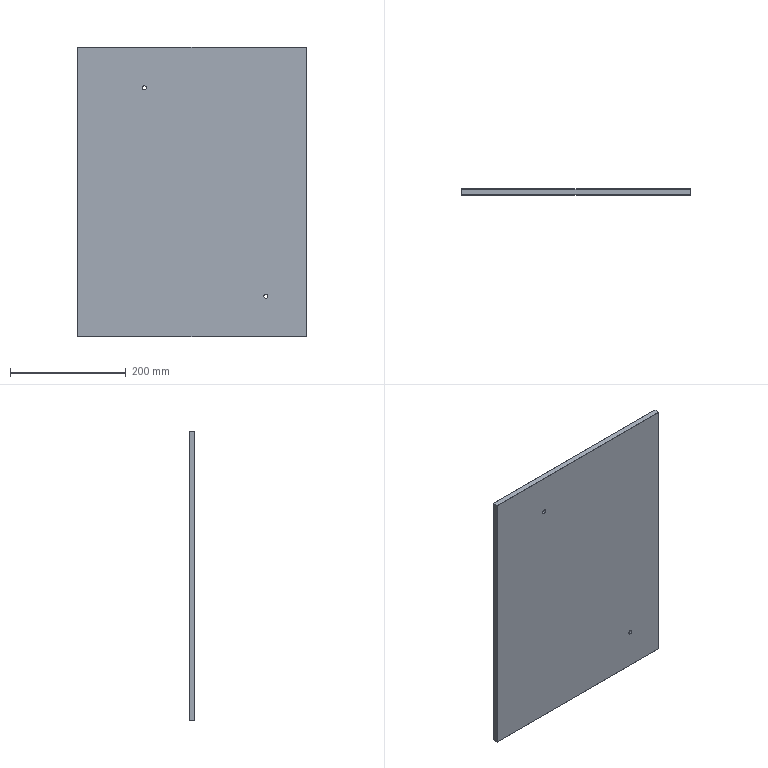Part | NX | 1 solid | 26 faces | box 395 x 10 x 500 mm | volume 1974067 mm3 | plane 18 | cylinder 4 | cone 4 | commonest cylinder face diameters 7 x4
STEP:
#1=CARTESIAN_POINT('',(374.7,0.,39.7));
#2=VERTEX_POINT('',#1);
#3=CARTESIAN_POINT('',(374.7,0.,-459.7));
#4=VERTEX_POINT('',#3);
#5=CARTESIAN_POINT('',(374.7,0.,-210.));
#6=DIRECTION('',(0.,0.,-1.));
#7=VECTOR('',#6,1000.);
#8=LINE('',#5,#7);
#9=EDGE_CURVE('',#2,#4,#8,.T.);
#10=ORIENTED_EDGE('',*,*,#9,.F.);
#11=CARTESIAN_POINT('',(-19.7,0.,39.7));
#12=VERTEX_POINT('',#11);
#13=CARTESIAN_POINT('',(177.5,0.,39.7));
#14=DIRECTION('',(-1.,0.,0.));
#15=VECTOR('',#14,1000.);
#16=LINE('',#13,#15);
#17=EDGE_CURVE('',#2,#12,#16,.T.);
#18=ORIENTED_EDGE('',*,*,#17,.T.);
#19=CARTESIAN_POINT('',(-19.7,0.,-459.7));
#20=VERTEX_POINT('',#19);
#21=CARTESIAN_POINT('',(-19.7,0.,-210.));
#22=DIRECTION('',(0.,0.,1.));
#23=VECTOR('',#22,1000.);
#24=LINE('',#21,#23);
#25=EDGE_CURVE('',#20,#12,#24,.T.);
#26=ORIENTED_EDGE('',*,*,#25,.F.);
#27=CARTESIAN_POINT('',(177.5,0.,-459.7));
#28=DIRECTION('',(1.,0.,0.));
#29=VECTOR('',#28,1000.);
#30=LINE('',#27,#29);
#31=EDGE_CURVE('',#20,#4,#30,.T.);
#32=ORIENTED_EDGE('',*,*,#31,.T.);
#33=EDGE_LOOP('',(#10,#18,#26,#32));
#34=FACE_BOUND('',#33,.T.);
#35=CARTESIAN_POINT('',(301.5,0.,-390.));
#36=VERTEX_POINT('',#35);
#37=CARTESIAN_POINT('',(308.5,0.,-390.));
#38=VERTEX_POINT('',#37);
#39=CARTESIAN_POINT('',(305.,0.,-390.));
#40=DIRECTION('',(0.,1.,0.));
#41=DIRECTION('',(1.,0.,0.));
#42=AXIS2_PLACEMENT_3D('',#39,#40,#41);
#43=CIRCLE('',#42,3.5);
#44=EDGE_CURVE('',#36,#38,#43,.T.);
#45=ORIENTED_EDGE('',*,*,#44,.T.);
#46=CARTESIAN_POINT('',(305.,0.,-390.));
#47=DIRECTION('',(0.,1.,0.));
#48=DIRECTION('',(1.,0.,0.));
#49=AXIS2_PLACEMENT_3D('',#46,#47,#48);
#50=CIRCLE('',#49,3.5);
#51=EDGE_CURVE('',#38,#36,#50,.T.);
#52=ORIENTED_EDGE('',*,*,#51,.T.);
#53=EDGE_LOOP('',(#45,#52));
#54=FACE_BOUND('',#53,.T.);
#55=CARTESIAN_POINT('',(91.5,0.,-30.));
#56=VERTEX_POINT('',#55);
#57=CARTESIAN_POINT('',(98.5,0.,-30.));
#58=VERTEX_POINT('',#57);
#59=CARTESIAN_POINT('',(95.,0.,-30.));
#60=DIRECTION('',(0.,1.,0.));
#61=DIRECTION('',(1.,0.,0.));
#62=AXIS2_PLACEMENT_3D('',#59,#60,#61);
#63=CIRCLE('',#62,3.5);
#64=EDGE_CURVE('',#56,#58,#63,.T.);
#65=ORIENTED_EDGE('',*,*,#64,.T.);
#66=CARTESIAN_POINT('',(95.,0.,-30.));
#67=DIRECTION('',(0.,1.,0.));
#68=DIRECTION('',(1.,0.,0.));
#69=AXIS2_PLACEMENT_3D('',#66,#67,#68);
#70=CIRCLE('',#69,3.5);
#71=EDGE_CURVE('',#58,#56,#70,.T.);
#72=ORIENTED_EDGE('',*,*,#71,.T.);
#73=EDGE_LOOP('',(#65,#72));
#74=FACE_BOUND('',#73,.T.);
#75=CARTESIAN_POINT('',(0.,0.,0.));
#76=DIRECTION('',(0.,1.,0.));
#77=DIRECTION('',(1.,0.,0.));
#78=AXIS2_PLACEMENT_3D('',#75,#76,#77);
#79=PLANE('',#78);
#80=ADVANCED_FACE('',(#34,#54,#74),#79,.F.);
#81=CARTESIAN_POINT('',(374.7,9.7,40.));
#82=VERTEX_POINT('',#81);
#83=CARTESIAN_POINT('',(374.7,0.3,40.));
#84=VERTEX_POINT('',#83);
#85=CARTESIAN_POINT('',(374.7,5.,40.));
#86=DIRECTION('',(0.,-1.,0.));
#87=VECTOR('',#86,1000.);
#88=LINE('',#85,#87);
#89=EDGE_CURVE('',#82,#84,#88,.T.);
#90=ORIENTED_EDGE('',*,*,#89,.F.);
#91=CARTESIAN_POINT('',(-19.7,9.7,40.));
#92=VERTEX_POINT('',#91);
#93=CARTESIAN_POINT('',(177.5,9.7,40.));
#94=DIRECTION('',(-1.,0.,0.));
#95=VECTOR('',#94,1000.);
#96=LINE('',#93,#95);
#97=EDGE_CURVE('',#82,#92,#96,.T.);
#98=ORIENTED_EDGE('',*,*,#97,.T.);
#99=CARTESIAN_POINT('',(-19.7,0.3,40.));
#100=VERTEX_POINT('',#99);
#101=CARTESIAN_POINT('',(-19.7,5.,40.));
#102=DIRECTION('',(0.,-1.,0.));
#103=VECTOR('',#102,1000.);
#104=LINE('',#101,#103);
#105=EDGE_CURVE('',#92,#100,#104,.T.);
#106=ORIENTED_EDGE('',*,*,#105,.T.);
#107=CARTESIAN_POINT('',(177.5,0.3,40.));
#108=DIRECTION('',(-1.,0.,0.));
#109=VECTOR('',#108,1000.);
#110=LINE('',#107,#109);
#111=EDGE_CURVE('',#84,#100,#110,.T.);
#112=ORIENTED_EDGE('',*,*,#111,.F.);
#113=EDGE_LOOP('',(#90,#98,#106,#112));
#114=FACE_BOUND('',#113,.T.);
#115=CARTESIAN_POINT('',(-80.,-56.,40.));
#116=DIRECTION('',(0.,0.,-1.));
#117=DIRECTION('',(0.,-1.,0.));
#118=AXIS2_PLACEMENT_3D('',#115,#116,#117);
#119=PLANE('',#118);
#120=ADVANCED_FACE('',(#114),#119,.F.);
#121=CARTESIAN_POINT('',(374.7,10.,39.7));
#122=VERTEX_POINT('',#121);
#123=CARTESIAN_POINT('',(374.7,10.,-459.7));
#124=VERTEX_POINT('',#123);
#125=CARTESIAN_POINT('',(374.7,10.,-210.));
#126=DIRECTION('',(0.,0.,-1.));
#127=VECTOR('',#126,1000.);
#128=LINE('',#125,#127);
#129=EDGE_CURVE('',#122,#124,#128,.T.);
#130=ORIENTED_EDGE('',*,*,#129,.T.);
#131=CARTESIAN_POINT('',(-19.7,10.,-459.7));
#132=VERTEX_POINT('',#131);
#133=CARTESIAN_POINT('',(177.5,10.,-459.7));
#134=DIRECTION('',(1.,0.,0.));
#135=VECTOR('',#134,1000.);
#136=LINE('',#133,#135);
#137=EDGE_CURVE('',#132,#124,#136,.T.);
#138=ORIENTED_EDGE('',*,*,#137,.F.);
#139=CARTESIAN_POINT('',(-19.7,10.,39.7));
#140=VERTEX_POINT('',#139);
#141=CARTESIAN_POINT('',(-19.7,10.,-210.));
#142=DIRECTION('',(0.,0.,1.));
#143=VECTOR('',#142,1000.);
#144=LINE('',#141,#143);
#145=EDGE_CURVE('',#132,#140,#144,.T.);
#146=ORIENTED_EDGE('',*,*,#145,.T.);
#147=CARTESIAN_POINT('',(177.5,10.,39.7));
#148=DIRECTION('',(-1.,0.,0.));
#149=VECTOR('',#148,1000.);
#150=LINE('',#147,#149);
#151=EDGE_CURVE('',#122,#140,#150,.T.);
#152=ORIENTED_EDGE('',*,*,#151,.F.);
#153=EDGE_LOOP('',(#130,#138,#146,#152));
#154=FACE_BOUND('',#153,.T.);
#155=CARTESIAN_POINT('',(91.3,10.,-30.));
#156=VERTEX_POINT('',#155);
#157=CARTESIAN_POINT('',(98.7,10.,-30.));
#158=VERTEX_POINT('',#157);
#159=CARTESIAN_POINT('',(95.,10.,-30.));
#160=DIRECTION('',(0.,1.,0.));
#161=DIRECTION('',(1.,0.,0.));
#162=AXIS2_PLACEMENT_3D('',#159,#160,#161);
#163=CIRCLE('',#162,3.7);
#164=EDGE_CURVE('',#156,#158,#163,.T.);
#165=ORIENTED_EDGE('',*,*,#164,.F.);
#166=CARTESIAN_POINT('',(95.,10.,-30.));
#167=DIRECTION('',(0.,1.,0.));
#168=DIRECTION('',(1.,0.,0.));
#169=AXIS2_PLACEMENT_3D('',#166,#167,#168);
#170=CIRCLE('',#169,3.7);
#171=EDGE_CURVE('',#158,#156,#170,.T.);
#172=ORIENTED_EDGE('',*,*,#171,.F.);
#173=EDGE_LOOP('',(#165,#172));
#174=FACE_BOUND('',#173,.T.);
#175=CARTESIAN_POINT('',(301.3,10.,-390.));
#176=VERTEX_POINT('',#175);
#177=CARTESIAN_POINT('',(308.7,10.,-390.));
#178=VERTEX_POINT('',#177);
#179=CARTESIAN_POINT('',(305.,10.,-390.));
#180=DIRECTION('',(0.,1.,0.));
#181=DIRECTION('',(1.,0.,0.));
#182=AXIS2_PLACEMENT_3D('',#179,#180,#181);
#183=CIRCLE('',#182,3.7);
#184=EDGE_CURVE('',#176,#178,#183,.T.);
#185=ORIENTED_EDGE('',*,*,#184,.F.);
#186=CARTESIAN_POINT('',(305.,10.,-390.));
#187=DIRECTION('',(0.,1.,0.));
#188=DIRECTION('',(1.,0.,0.));
#189=AXIS2_PLACEMENT_3D('',#186,#187,#188);
#190=CIRCLE('',#189,3.7);
#191=EDGE_CURVE('',#178,#176,#190,.T.);
#192=ORIENTED_EDGE('',*,*,#191,.F.);
#193=EDGE_LOOP('',(#185,#192));
#194=FACE_BOUND('',#193,.T.);
#195=CARTESIAN_POINT('',(0.,10.,0.));
#196=DIRECTION('',(0.,1.,0.));
#197=DIRECTION('',(1.,0.,0.));
#198=AXIS2_PLACEMENT_3D('',#195,#196,#197);
#199=PLANE('',#198);
#200=ADVANCED_FACE('',(#154,#174,#194),#199,.T.);
#201=CARTESIAN_POINT('',(-20.,0.3,-459.7));
#202=VERTEX_POINT('',#201);
#203=CARTESIAN_POINT('',(-20.,0.3,39.7));
#204=VERTEX_POINT('',#203);
#205=CARTESIAN_POINT('',(-20.,0.3,-210.));
#206=DIRECTION('',(0.,0.,1.));
#207=VECTOR('',#206,1000.);
#208=LINE('',#205,#207);
#209=EDGE_CURVE('',#202,#204,#208,.T.);
#210=ORIENTED_EDGE('',*,*,#209,.T.);
#211=CARTESIAN_POINT('',(-20.,9.7,39.7));
#212=VERTEX_POINT('',#211);
#213=CARTESIAN_POINT('',(-20.,5.,39.7));
#214=DIRECTION('',(0.,-1.,0.));
#215=VECTOR('',#214,1000.);
#216=LINE('',#213,#215);
#217=EDGE_CURVE('',#212,#204,#216,.T.);
#218=ORIENTED_EDGE('',*,*,#217,.F.);
#219=CARTESIAN_POINT('',(-20.,9.7,-459.7));
#220=VERTEX_POINT('',#219);
#221=CARTESIAN_POINT('',(-20.,9.7,-210.));
#222=DIRECTION('',(0.,0.,1.));
#223=VECTOR('',#222,1000.);
#224=LINE('',#221,#223);
#225=EDGE_CURVE('',#220,#212,#224,.T.);
#226=ORIENTED_EDGE('',*,*,#225,.F.);
#227=CARTESIAN_POINT('',(-20.,5.,-459.7));
#228=DIRECTION('',(0.,1.,0.));
#229=VECTOR('',#228,1000.);
#230=LINE('',#227,#229);
#231=EDGE_CURVE('',#202,#220,#230,.T.);
#232=ORIENTED_EDGE('',*,*,#231,.F.);
#233=EDGE_LOOP('',(#210,#218,#226,#232));
#234=FACE_BOUND('',#233,.T.);
#235=CARTESIAN_POINT('',(-20.,0.,-320.));
#236=DIRECTION('',(-1.,0.,0.));
#237=DIRECTION('',(0.,0.,1.));
#238=AXIS2_PLACEMENT_3D('',#235,#236,#237);
#239=PLANE('',#238);
#240=ADVANCED_FACE('',(#234),#239,.T.);
#241=CARTESIAN_POINT('',(375.,0.3,39.7));
#242=VERTEX_POINT('',#241);
#243=CARTESIAN_POINT('',(375.,0.3,-459.7));
#244=VERTEX_POINT('',#243);
#245=CARTESIAN_POINT('',(375.,0.3,-210.));
#246=DIRECTION('',(0.,0.,-1.));
#247=VECTOR('',#246,1000.);
#248=LINE('',#245,#247);
#249=EDGE_CURVE('',#242,#244,#248,.T.);
#250=ORIENTED_EDGE('',*,*,#249,.T.);
#251=CARTESIAN_POINT('',(375.,9.7,-459.7));
#252=VERTEX_POINT('',#251);
#253=CARTESIAN_POINT('',(375.,5.,-459.7));
#254=DIRECTION('',(0.,1.,0.));
#255=VECTOR('',#254,1000.);
#256=LINE('',#253,#255);
#257=EDGE_CURVE('',#244,#252,#256,.T.);
#258=ORIENTED_EDGE('',*,*,#257,.T.);
#259=CARTESIAN_POINT('',(375.,9.7,39.7));
#260=VERTEX_POINT('',#259);
#261=CARTESIAN_POINT('',(375.,9.7,-210.));
#262=DIRECTION('',(0.,0.,-1.));
#263=VECTOR('',#262,1000.);
#264=LINE('',#261,#263);
#265=EDGE_CURVE('',#260,#252,#264,.T.);
#266=ORIENTED_EDGE('',*,*,#265,.F.);
#267=CARTESIAN_POINT('',(375.,5.,39.7));
#268=DIRECTION('',(0.,-1.,0.));
#269=VECTOR('',#268,1000.);
#270=LINE('',#267,#269);
#271=EDGE_CURVE('',#260,#242,#270,.T.);
#272=ORIENTED_EDGE('',*,*,#271,.T.);
#273=EDGE_LOOP('',(#250,#258,#266,#272));
#274=FACE_BOUND('',#273,.T.);
#275=CARTESIAN_POINT('',(375.,0.,0.));
#276=DIRECTION('',(1.,0.,0.));
#277=DIRECTION('',(0.,1.,0.));
#278=AXIS2_PLACEMENT_3D('',#275,#276,#277);
#279=PLANE('',#278);
#280=ADVANCED_FACE('',(#274),#279,.T.);
#281=CARTESIAN_POINT('',(374.7,0.3,-460.));
#282=VERTEX_POINT('',#281);
#283=CARTESIAN_POINT('',(374.7,9.7,-460.));
#284=VERTEX_POINT('',#283);
#285=CARTESIAN_POINT('',(374.7,5.,-460.));
#286=DIRECTION('',(0.,1.,0.));
#287=VECTOR('',#286,1000.);
#288=LINE('',#285,#287);
#289=EDGE_CURVE('',#282,#284,#288,.T.);
#290=ORIENTED_EDGE('',*,*,#289,.F.);
#291=CARTESIAN_POINT('',(-19.7,0.3,-460.));
#292=VERTEX_POINT('',#291);
#293=CARTESIAN_POINT('',(177.5,0.3,-460.));
#294=DIRECTION('',(1.,0.,0.));
#295=VECTOR('',#294,1000.);
#296=LINE('',#293,#295);
#297=EDGE_CURVE('',#292,#282,#296,.T.);
#298=ORIENTED_EDGE('',*,*,#297,.F.);
#299=CARTESIAN_POINT('',(-19.7,9.7,-460.));
#300=VERTEX_POINT('',#299);
#301=CARTESIAN_POINT('',(-19.7,5.,-460.));
#302=DIRECTION('',(0.,1.,0.));
#303=VECTOR('',#302,1000.);
#304=LINE('',#301,#303);
#305=EDGE_CURVE('',#292,#300,#304,.T.);
#306=ORIENTED_EDGE('',*,*,#305,.T.);
#307=CARTESIAN_POINT('',(177.5,9.7,-460.));
#308=DIRECTION('',(1.,0.,0.));
#309=VECTOR('',#308,1000.);
#310=LINE('',#307,#309);
#311=EDGE_CURVE('',#300,#284,#310,.T.);
#312=ORIENTED_EDGE('',*,*,#311,.T.);
#313=EDGE_LOOP('',(#290,#298,#306,#312));
#314=FACE_BOUND('',#313,.T.);
#315=CARTESIAN_POINT('',(350.,-56.,-460.));
#316=DIRECTION('',(0.,0.,1.));
#317=DIRECTION('',(1.,0.,0.));
#318=AXIS2_PLACEMENT_3D('',#315,#316,#317);
#319=PLANE('',#318);
#320=ADVANCED_FACE('',(#314),#319,.F.);
#321=CARTESIAN_POINT('',(301.5,9.8,-390.));
#322=VERTEX_POINT('',#321);
#323=CARTESIAN_POINT('',(308.5,9.8,-390.));
#324=VERTEX_POINT('',#323);
#325=CARTESIAN_POINT('',(305.,9.8,-390.));
#326=DIRECTION('',(0.,1.,0.));
#327=DIRECTION('',(1.,0.,0.));
#328=AXIS2_PLACEMENT_3D('',#325,#326,#327);
#329=CIRCLE('',#328,3.5);
#330=EDGE_CURVE('',#322,#324,#329,.T.);
#331=ORIENTED_EDGE('',*,*,#330,.T.);
#332=CARTESIAN_POINT('',(308.5,10.,-390.));
#333=DIRECTION('',(0.,1.,0.));
#334=VECTOR('',#333,1000.);
#335=LINE('',#332,#334);
#336=EDGE_CURVE('',#38,#324,#335,.T.);
#337=ORIENTED_EDGE('',*,*,#336,.F.);
#338=ORIENTED_EDGE('',*,*,#44,.F.);
#339=CARTESIAN_POINT('',(301.5,10.,-390.));
#340=DIRECTION('',(0.,1.,0.));
#341=VECTOR('',#340,1000.);
#342=LINE('',#339,#341);
#343=EDGE_CURVE('',#36,#322,#342,.T.);
#344=ORIENTED_EDGE('',*,*,#343,.T.);
#345=EDGE_LOOP('',(#331,#337,#338,#344));
#346=FACE_BOUND('',#345,.T.);
#347=CARTESIAN_POINT('',(305.,10.,-390.));
#348=DIRECTION('',(0.,1.,0.));
#349=DIRECTION('',(1.,0.,0.));
#350=AXIS2_PLACEMENT_3D('',#347,#348,#349);
#351=CYLINDRICAL_SURFACE('',#350,3.5);
#352=ADVANCED_FACE('',(#346),#351,.F.);
#353=ORIENTED_EDGE('',*,*,#330,.F.);
#354=CARTESIAN_POINT('',(301.5,9.8,-390.));
#355=DIRECTION('',(-0.7071,0.7071,0.));
#356=VECTOR('',#355,1000.);
#357=LINE('',#354,#356);
#358=EDGE_CURVE('',#322,#176,#357,.T.);
#359=ORIENTED_EDGE('',*,*,#358,.T.);
#360=ORIENTED_EDGE('',*,*,#184,.T.);
#361=CARTESIAN_POINT('',(308.5,9.8,-390.));
#362=DIRECTION('',(0.7071,0.7071,0.));
#363=VECTOR('',#362,1000.);
#364=LINE('',#361,#363);
#365=EDGE_CURVE('',#324,#178,#364,.T.);
#366=ORIENTED_EDGE('',*,*,#365,.F.);
#367=EDGE_LOOP('',(#353,#359,#360,#366));
#368=FACE_BOUND('',#367,.T.);
#369=CARTESIAN_POINT('',(305.,9.8,-390.));
#370=DIRECTION('',(0.,1.,0.));
#371=DIRECTION('',(1.,0.,0.));
#372=AXIS2_PLACEMENT_3D('',#369,#370,#371);
#373=CONICAL_SURFACE('',#372,3.5,0.7854);
#374=ADVANCED_FACE('',(#368),#373,.F.);
#375=CARTESIAN_POINT('',(91.5,9.8,-30.));
#376=VERTEX_POINT('',#375);
#377=CARTESIAN_POINT('',(98.5,9.8,-30.));
#378=VERTEX_POINT('',#377);
#379=CARTESIAN_POINT('',(95.,9.8,-30.));
#380=DIRECTION('',(0.,1.,0.));
#381=DIRECTION('',(1.,0.,0.));
#382=AXIS2_PLACEMENT_3D('',#379,#380,#381);
#383=CIRCLE('',#382,3.5);
#384=EDGE_CURVE('',#376,#378,#383,.T.);
#385=ORIENTED_EDGE('',*,*,#384,.T.);
#386=CARTESIAN_POINT('',(98.5,10.,-30.));
#387=DIRECTION('',(0.,1.,0.));
#388=VECTOR('',#387,1000.);
#389=LINE('',#386,#388);
#390=EDGE_CURVE('',#58,#378,#389,.T.);
#391=ORIENTED_EDGE('',*,*,#390,.F.);
#392=ORIENTED_EDGE('',*,*,#64,.F.);
#393=CARTESIAN_POINT('',(91.5,10.,-30.));
#394=DIRECTION('',(0.,1.,0.));
#395=VECTOR('',#394,1000.);
#396=LINE('',#393,#395);
#397=EDGE_CURVE('',#56,#376,#396,.T.);
#398=ORIENTED_EDGE('',*,*,#397,.T.);
#399=EDGE_LOOP('',(#385,#391,#392,#398));
#400=FACE_BOUND('',#399,.T.);
#401=CARTESIAN_POINT('',(95.,10.,-30.));
#402=DIRECTION('',(0.,1.,0.));
#403=DIRECTION('',(1.,0.,0.));
#404=AXIS2_PLACEMENT_3D('',#401,#402,#403);
#405=CYLINDRICAL_SURFACE('',#404,3.5);
#406=ADVANCED_FACE('',(#400),#405,.F.);
#407=ORIENTED_EDGE('',*,*,#384,.F.);
#408=CARTESIAN_POINT('',(91.5,9.8,-30.));
#409=DIRECTION('',(-0.7071,0.7071,0.));
#410=VECTOR('',#409,1000.);
#411=LINE('',#408,#410);
#412=EDGE_CURVE('',#376,#156,#411,.T.);
#413=ORIENTED_EDGE('',*,*,#412,.T.);
#414=ORIENTED_EDGE('',*,*,#164,.T.);
#415=CARTESIAN_POINT('',(98.5,9.8,-30.));
#416=DIRECTION('',(0.7071,0.7071,0.));
#417=VECTOR('',#416,1000.);
#418=LINE('',#415,#417);
#419=EDGE_CURVE('',#378,#158,#418,.T.);
#420=ORIENTED_EDGE('',*,*,#419,.F.);
#421=EDGE_LOOP('',(#407,#413,#414,#420));
#422=FACE_BOUND('',#421,.T.);
#423=CARTESIAN_POINT('',(95.,9.8,-30.));
#424=DIRECTION('',(0.,1.,0.));
#425=DIRECTION('',(1.,0.,0.));
#426=AXIS2_PLACEMENT_3D('',#423,#424,#425);
#427=CONICAL_SURFACE('',#426,3.5,0.7854);
#428=ADVANCED_FACE('',(#422),#427,.F.);
#429=ORIENTED_EDGE('',*,*,#151,.T.);
#430=CARTESIAN_POINT('',(-19.85,9.85,39.85));
#431=VERTEX_POINT('',#430);
#432=CARTESIAN_POINT('',(20.,49.7,0.));
#433=DIRECTION('',(0.5774,0.5774,-0.5774));
#434=VECTOR('',#433,1000.);
#435=LINE('',#432,#434);
#436=EDGE_CURVE('',#431,#140,#435,.T.);
#437=ORIENTED_EDGE('',*,*,#436,.F.);
#438=CARTESIAN_POINT('',(-59.7,49.7,0.));
#439=DIRECTION('',(-0.5774,0.5774,-0.5774));
#440=VECTOR('',#439,1000.);
#441=LINE('',#438,#440);
#442=EDGE_CURVE('',#92,#431,#441,.T.);
#443=ORIENTED_EDGE('',*,*,#442,.F.);
#444=ORIENTED_EDGE('',*,*,#97,.F.);
#445=CARTESIAN_POINT('',(374.85,9.85,39.85));
#446=VERTEX_POINT('',#445);
#447=CARTESIAN_POINT('',(0.,-365.,414.7));
#448=DIRECTION('',(-0.5774,-0.5774,0.5774));
#449=VECTOR('',#448,1000.);
#450=LINE('',#447,#449);
#451=EDGE_CURVE('',#446,#82,#450,.T.);
#452=ORIENTED_EDGE('',*,*,#451,.F.);
#453=CARTESIAN_POINT('',(0.,384.7,-335.));
#454=DIRECTION('',(-0.5774,0.5774,-0.5774));
#455=VECTOR('',#454,1000.);
#456=LINE('',#453,#455);
#457=EDGE_CURVE('',#446,#122,#456,.T.);
#458=ORIENTED_EDGE('',*,*,#457,.T.);
#459=EDGE_LOOP('',(#429,#437,#443,#444,#452,#458));
#460=FACE_BOUND('',#459,.T.);
#461=CARTESIAN_POINT('',(177.5,9.85,39.85));
#462=DIRECTION('',(0.,-0.7071,-0.7071));
#463=DIRECTION('',(0.,-0.7071,0.7071));
#464=AXIS2_PLACEMENT_3D('',#461,#462,#463);
#465=PLANE('',#464);
#466=ADVANCED_FACE('',(#460),#465,.F.);
#467=ORIENTED_EDGE('',*,*,#105,.F.);
#468=ORIENTED_EDGE('',*,*,#442,.T.);
#469=CARTESIAN_POINT('',(-59.7,-30.,0.));
#470=DIRECTION('',(-0.5774,-0.5774,-0.5774));
#471=VECTOR('',#470,1000.);
#472=LINE('',#469,#471);
#473=EDGE_CURVE('',#431,#212,#472,.T.);
#474=ORIENTED_EDGE('',*,*,#473,.T.);
#475=ORIENTED_EDGE('',*,*,#217,.T.);
#476=CARTESIAN_POINT('',(-19.85,0.15,39.85));
#477=VERTEX_POINT('',#476);
#478=CARTESIAN_POINT('',(-59.7,40.,0.));
#479=DIRECTION('',(-0.5774,0.5774,-0.5774));
#480=VECTOR('',#479,1000.);
#481=LINE('',#478,#480);
#482=EDGE_CURVE('',#477,#204,#481,.T.);
#483=ORIENTED_EDGE('',*,*,#482,.F.);
#484=CARTESIAN_POINT('',(-59.7,-39.7,0.));
#485=DIRECTION('',(-0.5774,-0.5774,-0.5774));
#486=VECTOR('',#485,1000.);
#487=LINE('',#484,#486);
#488=EDGE_CURVE('',#100,#477,#487,.T.);
#489=ORIENTED_EDGE('',*,*,#488,.F.);
#490=EDGE_LOOP('',(#467,#468,#474,#475,#483,#489));
#491=FACE_BOUND('',#490,.T.);
#492=CARTESIAN_POINT('',(-19.85,5.,39.85));
#493=DIRECTION('',(-0.7071,0.,0.7071));
#494=DIRECTION('',(0.,1.,0.));
#495=AXIS2_PLACEMENT_3D('',#492,#493,#494);
#496=PLANE('',#495);
#497=ADVANCED_FACE('',(#491),#496,.T.);
#498=ORIENTED_EDGE('',*,*,#145,.F.);
#499=CARTESIAN_POINT('',(-19.85,9.85,-459.85));
#500=VERTEX_POINT('',#499);
#501=CARTESIAN_POINT('',(440.,469.7,0.));
#502=DIRECTION('',(-0.5774,-0.5774,-0.5774));
#503=VECTOR('',#502,1000.);
#504=LINE('',#501,#503);
#505=EDGE_CURVE('',#132,#500,#504,.T.);
#506=ORIENTED_EDGE('',*,*,#505,.T.);
#507=CARTESIAN_POINT('',(-479.7,-450.,0.));
#508=DIRECTION('',(-0.5774,-0.5774,0.5774));
#509=VECTOR('',#508,1000.);
#510=LINE('',#507,#509);
#511=EDGE_CURVE('',#500,#220,#510,.T.);
#512=ORIENTED_EDGE('',*,*,#511,.T.);
#513=ORIENTED_EDGE('',*,*,#225,.T.);
#514=ORIENTED_EDGE('',*,*,#473,.F.);
#515=ORIENTED_EDGE('',*,*,#436,.T.);
#516=EDGE_LOOP('',(#498,#506,#512,#513,#514,#515));
#517=FACE_BOUND('',#516,.T.);
#518=CARTESIAN_POINT('',(-19.85,9.85,-210.));
#519=DIRECTION('',(-0.7071,0.7071,0.));
#520=DIRECTION('',(0.,0.,1.));
#521=AXIS2_PLACEMENT_3D('',#518,#519,#520);
#522=PLANE('',#521);
#523=ADVANCED_FACE('',(#517),#522,.T.);
#524=ORIENTED_EDGE('',*,*,#25,.T.);
#525=CARTESIAN_POINT('',(0.,-19.7,20.));
#526=DIRECTION('',(-0.5774,0.5774,0.5774));
#527=VECTOR('',#526,1000.);
#528=LINE('',#525,#527);
#529=EDGE_CURVE('',#12,#477,#528,.T.);
#530=ORIENTED_EDGE('',*,*,#529,.T.);
#531=ORIENTED_EDGE('',*,*,#482,.T.);
#532=ORIENTED_EDGE('',*,*,#209,.F.);
#533=CARTESIAN_POINT('',(-19.85,0.15,-459.85));
#534=VERTEX_POINT('',#533);
#535=CARTESIAN_POINT('',(-479.7,460.,0.));
#536=DIRECTION('',(-0.5774,0.5774,0.5774));
#537=VECTOR('',#536,1000.);
#538=LINE('',#535,#537);
#539=EDGE_CURVE('',#534,#202,#538,.T.);
#540=ORIENTED_EDGE('',*,*,#539,.F.);
#541=CARTESIAN_POINT('',(440.,-459.7,0.));
#542=DIRECTION('',(0.5774,-0.5774,0.5774));
#543=VECTOR('',#542,1000.);
#544=LINE('',#541,#543);
#545=EDGE_CURVE('',#534,#20,#544,.T.);
#546=ORIENTED_EDGE('',*,*,#545,.T.);
#547=EDGE_LOOP('',(#524,#530,#531,#532,#540,#546));
#548=FACE_BOUND('',#547,.T.);
#549=CARTESIAN_POINT('',(-19.85,0.15,-210.));
#550=DIRECTION('',(0.7071,0.7071,0.));
#551=DIRECTION('',(0.,0.,-1.));
#552=AXIS2_PLACEMENT_3D('',#549,#550,#551);
#553=PLANE('',#552);
#554=ADVANCED_FACE('',(#548),#553,.F.);
#555=ORIENTED_EDGE('',*,*,#111,.T.);
#556=ORIENTED_EDGE('',*,*,#488,.T.);
#557=ORIENTED_EDGE('',*,*,#529,.F.);
#558=ORIENTED_EDGE('',*,*,#17,.F.);
#559=CARTESIAN_POINT('',(374.85,0.15,39.85));
#560=VERTEX_POINT('',#559);
#561=CARTESIAN_POINT('',(0.,-374.7,-335.));
#562=DIRECTION('',(-0.5774,-0.5774,-0.5774));
#563=VECTOR('',#562,1000.);
#564=LINE('',#561,#563);
#565=EDGE_CURVE('',#560,#2,#564,.T.);
#566=ORIENTED_EDGE('',*,*,#565,.F.);
#567=CARTESIAN_POINT('',(0.,375.,414.7));
#568=DIRECTION('',(0.5774,-0.5774,-0.5774));
#569=VECTOR('',#568,1000.);
#570=LINE('',#567,#569);
#571=EDGE_CURVE('',#84,#560,#570,.T.);
#572=ORIENTED_EDGE('',*,*,#571,.F.);
#573=EDGE_LOOP('',(#555,#556,#557,#558,#566,#572));
#574=FACE_BOUND('',#573,.T.);
#575=CARTESIAN_POINT('',(177.5,0.15,39.85));
#576=DIRECTION('',(0.,0.7071,-0.7071));
#577=DIRECTION('',(-1.,0.,0.));
#578=AXIS2_PLACEMENT_3D('',#575,#576,#577);
#579=PLANE('',#578);
#580=ADVANCED_FACE('',(#574),#579,.F.);
#581=ORIENTED_EDGE('',*,*,#311,.F.);
#582=CARTESIAN_POINT('',(-479.7,469.7,0.));
#583=DIRECTION('',(-0.5774,0.5774,0.5774));
#584=VECTOR('',#583,1000.);
#585=LINE('',#582,#584);
#586=EDGE_CURVE('',#300,#500,#585,.T.);
#587=ORIENTED_EDGE('',*,*,#586,.T.);
#588=ORIENTED_EDGE('',*,*,#505,.F.);
#589=ORIENTED_EDGE('',*,*,#137,.T.);
#590=CARTESIAN_POINT('',(374.85,9.85,-459.85));
#591=VERTEX_POINT('',#590);
#592=CARTESIAN_POINT('',(-85.,469.7,0.));
#593=DIRECTION('',(-0.5774,0.5774,0.5774));
#594=VECTOR('',#593,1000.);
#595=LINE('',#592,#594);
#596=EDGE_CURVE('',#591,#124,#595,.T.);
#597=ORIENTED_EDGE('',*,*,#596,.F.);
#598=CARTESIAN_POINT('',(834.7,469.7,0.));
#599=DIRECTION('',(-0.5774,-0.5774,-0.5774));
#600=VECTOR('',#599,1000.);
#601=LINE('',#598,#600);
#602=EDGE_CURVE('',#591,#284,#601,.T.);
#603=ORIENTED_EDGE('',*,*,#602,.T.);
#604=EDGE_LOOP('',(#581,#587,#588,#589,#597,#603));
#605=FACE_BOUND('',#604,.T.);
#606=CARTESIAN_POINT('',(177.5,9.85,-459.85));
#607=DIRECTION('',(0.,0.7071,-0.7071));
#608=DIRECTION('',(-1.,0.,0.));
#609=AXIS2_PLACEMENT_3D('',#606,#607,#608);
#610=PLANE('',#609);
#611=ADVANCED_FACE('',(#605),#610,.T.);
#612=ORIENTED_EDGE('',*,*,#305,.F.);
#613=CARTESIAN_POINT('',(-479.7,-459.7,0.));
#614=DIRECTION('',(0.5774,0.5774,-0.5774));
#615=VECTOR('',#614,1000.);
#616=LINE('',#613,#615);
#617=EDGE_CURVE('',#534,#292,#616,.T.);
#618=ORIENTED_EDGE('',*,*,#617,.F.);
#619=ORIENTED_EDGE('',*,*,#539,.T.);
#620=ORIENTED_EDGE('',*,*,#231,.T.);
#621=ORIENTED_EDGE('',*,*,#511,.F.);
#622=ORIENTED_EDGE('',*,*,#586,.F.);
#623=EDGE_LOOP('',(#612,#618,#619,#620,#621,#622));
#624=FACE_BOUND('',#623,.T.);
#625=CARTESIAN_POINT('',(-19.85,5.,-459.85));
#626=DIRECTION('',(-0.7071,0.,-0.7071));
#627=DIRECTION('',(-0.7071,0.,0.7071));
#628=AXIS2_PLACEMENT_3D('',#625,#626,#627);
#629=PLANE('',#628);
#630=ADVANCED_FACE('',(#624),#629,.T.);
#631=ORIENTED_EDGE('',*,*,#297,.T.);
#632=CARTESIAN_POINT('',(374.85,0.15,-459.85));
#633=VERTEX_POINT('',#632);
#634=CARTESIAN_POINT('',(834.7,-459.7,0.));
#635=DIRECTION('',(-0.5774,0.5774,-0.5774));
#636=VECTOR('',#635,1000.);
#637=LINE('',#634,#636);
#638=EDGE_CURVE('',#633,#282,#637,.T.);
#639=ORIENTED_EDGE('',*,*,#638,.F.);
#640=CARTESIAN_POINT('',(-85.,-459.7,0.));
#641=DIRECTION('',(0.5774,0.5774,-0.5774));
#642=VECTOR('',#641,1000.);
#643=LINE('',#640,#642);
#644=EDGE_CURVE('',#4,#633,#643,.T.);
#645=ORIENTED_EDGE('',*,*,#644,.F.);
#646=ORIENTED_EDGE('',*,*,#31,.F.);
#647=ORIENTED_EDGE('',*,*,#545,.F.);
#648=ORIENTED_EDGE('',*,*,#617,.T.);
#649=EDGE_LOOP('',(#631,#639,#645,#646,#647,#648));
#650=FACE_BOUND('',#649,.T.);
#651=CARTESIAN_POINT('',(177.5,0.15,-459.85));
#652=DIRECTION('',(0.,0.7071,0.7071));
#653=DIRECTION('',(1.,0.,0.));
#654=AXIS2_PLACEMENT_3D('',#651,#652,#653);
#655=PLANE('',#654);
#656=ADVANCED_FACE('',(#650),#655,.F.);
#657=ORIENTED_EDGE('',*,*,#9,.T.);
#658=ORIENTED_EDGE('',*,*,#644,.T.);
#659=CARTESIAN_POINT('',(834.7,460.,0.));
#660=DIRECTION('',(-0.5774,-0.5774,-0.5774));
#661=VECTOR('',#660,1000.);
#662=LINE('',#659,#661);
#663=EDGE_CURVE('',#244,#633,#662,.T.);
#664=ORIENTED_EDGE('',*,*,#663,.F.);
#665=ORIENTED_EDGE('',*,*,#249,.F.);
#666=CARTESIAN_POINT('',(0.,-374.7,414.7));
#667=DIRECTION('',(0.5774,0.5774,-0.5774));
#668=VECTOR('',#667,1000.);
#669=LINE('',#666,#668);
#670=EDGE_CURVE('',#560,#242,#669,.T.);
#671=ORIENTED_EDGE('',*,*,#670,.F.);
#672=ORIENTED_EDGE('',*,*,#565,.T.);
#673=EDGE_LOOP('',(#657,#658,#664,#665,#671,#672));
#674=FACE_BOUND('',#673,.T.);
#675=CARTESIAN_POINT('',(374.85,0.15,-210.));
#676=DIRECTION('',(-0.7071,0.7071,0.));
#677=DIRECTION('',(0.,0.,1.));
#678=AXIS2_PLACEMENT_3D('',#675,#676,#677);
#679=PLANE('',#678);
#680=ADVANCED_FACE('',(#674),#679,.F.);
#681=ORIENTED_EDGE('',*,*,#89,.T.);
#682=ORIENTED_EDGE('',*,*,#571,.T.);
#683=ORIENTED_EDGE('',*,*,#670,.T.);
#684=ORIENTED_EDGE('',*,*,#271,.F.);
#685=CARTESIAN_POINT('',(0.,384.7,414.7));
#686=DIRECTION('',(-0.5774,0.5774,0.5774));
#687=VECTOR('',#686,1000.);
#688=LINE('',#685,#687);
#689=EDGE_CURVE('',#260,#446,#688,.T.);
#690=ORIENTED_EDGE('',*,*,#689,.T.);
#691=ORIENTED_EDGE('',*,*,#451,.T.);
#692=EDGE_LOOP('',(#681,#682,#683,#684,#690,#691));
#693=FACE_BOUND('',#692,.T.);
#694=CARTESIAN_POINT('',(374.85,5.,39.85));
#695=DIRECTION('',(-0.7071,0.,-0.7071));
#696=DIRECTION('',(-0.7071,0.,0.7071));
#697=AXIS2_PLACEMENT_3D('',#694,#695,#696);
#698=PLANE('',#697);
#699=ADVANCED_FACE('',(#693),#698,.F.);
#700=ORIENTED_EDGE('',*,*,#129,.F.);
#701=ORIENTED_EDGE('',*,*,#457,.F.);
#702=ORIENTED_EDGE('',*,*,#689,.F.);
#703=ORIENTED_EDGE('',*,*,#265,.T.);
#704=CARTESIAN_POINT('',(0.,384.7,-834.7));
#705=DIRECTION('',(-0.5774,0.5774,-0.5774));
#706=VECTOR('',#705,1000.);
#707=LINE('',#704,#706);
#708=EDGE_CURVE('',#252,#591,#707,.T.);
#709=ORIENTED_EDGE('',*,*,#708,.T.);
#710=ORIENTED_EDGE('',*,*,#596,.T.);
#711=EDGE_LOOP('',(#700,#701,#702,#703,#709,#710));
#712=FACE_BOUND('',#711,.T.);
#713=CARTESIAN_POINT('',(374.85,9.85,-210.));
#714=DIRECTION('',(0.7071,0.7071,0.));
#715=DIRECTION('',(0.,0.,-1.));
#716=AXIS2_PLACEMENT_3D('',#713,#714,#715);
#717=PLANE('',#716);
#718=ADVANCED_FACE('',(#712),#717,.T.);
#719=ORIENTED_EDGE('',*,*,#289,.T.);
#720=ORIENTED_EDGE('',*,*,#602,.F.);
#721=ORIENTED_EDGE('',*,*,#708,.F.);
#722=ORIENTED_EDGE('',*,*,#257,.F.);
#723=ORIENTED_EDGE('',*,*,#663,.T.);
#724=ORIENTED_EDGE('',*,*,#638,.T.);
#725=EDGE_LOOP('',(#719,#720,#721,#722,#723,#724));
#726=FACE_BOUND('',#725,.T.);
#727=CARTESIAN_POINT('',(374.85,5.,-459.85));
#728=DIRECTION('',(-0.7071,0.,0.7071));
#729=DIRECTION('',(0.,1.,0.));
#730=AXIS2_PLACEMENT_3D('',#727,#728,#729);
#731=PLANE('',#730);
#732=ADVANCED_FACE('',(#726),#731,.F.);
#733=ORIENTED_EDGE('',*,*,#390,.T.);
#734=CARTESIAN_POINT('',(95.,9.8,-30.));
#735=DIRECTION('',(0.,1.,0.));
#736=DIRECTION('',(1.,0.,0.));
#737=AXIS2_PLACEMENT_3D('',#734,#735,#736);
#738=CIRCLE('',#737,3.5);
#739=EDGE_CURVE('',#378,#376,#738,.T.);
#740=ORIENTED_EDGE('',*,*,#739,.T.);
#741=ORIENTED_EDGE('',*,*,#397,.F.);
#742=ORIENTED_EDGE('',*,*,#71,.F.);
#743=EDGE_LOOP('',(#733,#740,#741,#742));
#744=FACE_BOUND('',#743,.T.);
#745=CARTESIAN_POINT('',(95.,10.,-30.));
#746=DIRECTION('',(0.,1.,0.));
#747=DIRECTION('',(1.,0.,0.));
#748=AXIS2_PLACEMENT_3D('',#745,#746,#747);
#749=CYLINDRICAL_SURFACE('',#748,3.5);
#750=ADVANCED_FACE('',(#744),#749,.F.);
#751=ORIENTED_EDGE('',*,*,#419,.T.);
#752=ORIENTED_EDGE('',*,*,#171,.T.);
#753=ORIENTED_EDGE('',*,*,#412,.F.);
#754=ORIENTED_EDGE('',*,*,#739,.F.);
#755=EDGE_LOOP('',(#751,#752,#753,#754));
#756=FACE_BOUND('',#755,.T.);
#757=CARTESIAN_POINT('',(95.,9.8,-30.));
#758=DIRECTION('',(0.,1.,0.));
#759=DIRECTION('',(1.,0.,0.));
#760=AXIS2_PLACEMENT_3D('',#757,#758,#759);
#761=CONICAL_SURFACE('',#760,3.5,0.7854);
#762=ADVANCED_FACE('',(#756),#761,.F.);
#763=ORIENTED_EDGE('',*,*,#336,.T.);
#764=CARTESIAN_POINT('',(305.,9.8,-390.));
#765=DIRECTION('',(0.,1.,0.));
#766=DIRECTION('',(1.,0.,0.));
#767=AXIS2_PLACEMENT_3D('',#764,#765,#766);
#768=CIRCLE('',#767,3.5);
#769=EDGE_CURVE('',#324,#322,#768,.T.);
#770=ORIENTED_EDGE('',*,*,#769,.T.);
#771=ORIENTED_EDGE('',*,*,#343,.F.);
#772=ORIENTED_EDGE('',*,*,#51,.F.);
#773=EDGE_LOOP('',(#763,#770,#771,#772));
#774=FACE_BOUND('',#773,.T.);
#775=CARTESIAN_POINT('',(305.,10.,-390.));
#776=DIRECTION('',(0.,1.,0.));
#777=DIRECTION('',(1.,0.,0.));
#778=AXIS2_PLACEMENT_3D('',#775,#776,#777);
#779=CYLINDRICAL_SURFACE('',#778,3.5);
#780=ADVANCED_FACE('',(#774),#779,.F.);
#781=ORIENTED_EDGE('',*,*,#365,.T.);
#782=ORIENTED_EDGE('',*,*,#191,.T.);
#783=ORIENTED_EDGE('',*,*,#358,.F.);
#784=ORIENTED_EDGE('',*,*,#769,.F.);
#785=EDGE_LOOP('',(#781,#782,#783,#784));
#786=FACE_BOUND('',#785,.T.);
#787=CARTESIAN_POINT('',(305.,9.8,-390.));
#788=DIRECTION('',(0.,1.,0.));
#789=DIRECTION('',(1.,0.,0.));
#790=AXIS2_PLACEMENT_3D('',#787,#788,#789);
#791=CONICAL_SURFACE('',#790,3.5,0.7854);
#792=ADVANCED_FACE('',(#786),#791,.F.);
#793=CLOSED_SHELL('',(#80,#120,#200,#240,#280,#320,#352,#374,#406,#428,#466,#497,#523,#554,#580,#611,#630,#656,#680,#699,#718,#732,#750,#762,#780,#792));
#794=MANIFOLD_SOLID_BREP('',#793);
#795=(LENGTH_UNIT()NAMED_UNIT(*)SI_UNIT(.MILLI.,.METRE.));
#796=UNCERTAINTY_MEASURE_WITH_UNIT(LENGTH_MEASURE(0.00001),#795,'','');
#797=(NAMED_UNIT(*)PLANE_ANGLE_UNIT()SI_UNIT($,.RADIAN.));
#798=(NAMED_UNIT(*)SI_UNIT($,.STERADIAN.)SOLID_ANGLE_UNIT());
#799=(GEOMETRIC_REPRESENTATION_CONTEXT(3)GLOBAL_UNCERTAINTY_ASSIGNED_CONTEXT((#796))GLOBAL_UNIT_ASSIGNED_CONTEXT((#795,#797,#798))REPRESENTATION_CONTEXT('',''));
#800=ADVANCED_BREP_SHAPE_REPRESENTATION('',(#794),#799);